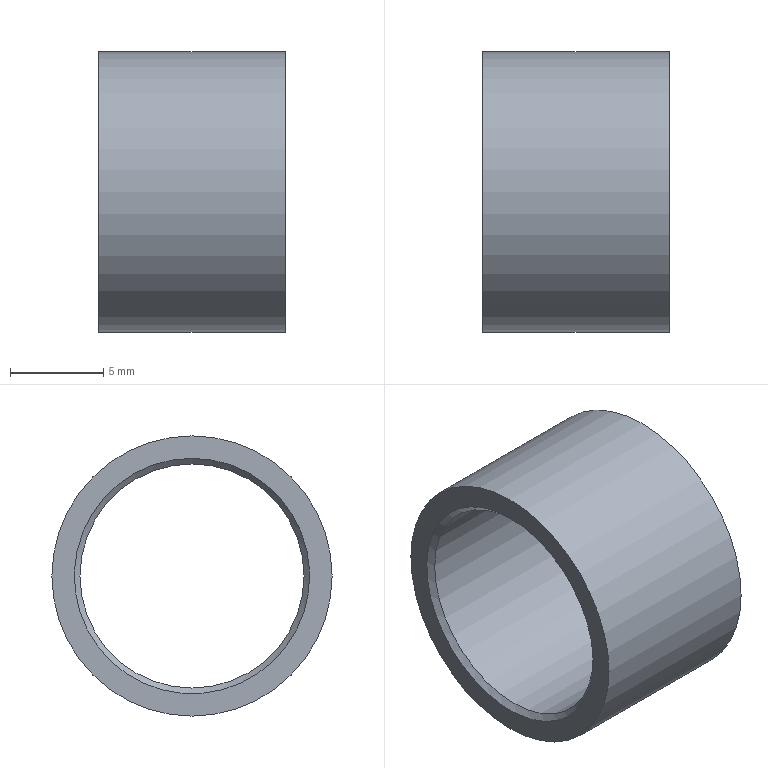Part | STEP file | 1 solid | 6 faces | box 10 x 15 x 15 mm | volume 632.723 mm3 | cylinder 2 | plane 2 | cone 2 | commonest cylinder face diameters 12 x1 15 x1
STEP:
#1=CARTESIAN_POINT('',(0.,0.,0.));
#2=DIRECTION('',(0.,0.,1.));
#3=DIRECTION('',(1.,0.,0.));
#4=AXIS2_PLACEMENT_3D('',#1,#2,#3);
#5=CARTESIAN_POINT('',(0.,0.,7.5));
#6=VERTEX_POINT('',#5);
#7=CARTESIAN_POINT('',(0.,0.,0.));
#8=DIRECTION('',(1.,0.,0.));
#9=DIRECTION('',(0.,0.,1.));
#10=AXIS2_PLACEMENT_3D('',#7,#8,#9);
#11=CIRCLE('',#10,7.5);
#12=CARTESIAN_POINT('',(0.,0.,0.));
#13=DIRECTION('',(-1.,0.,0.));
#14=DIRECTION('',(0.,0.,1.));
#15=AXIS2_PLACEMENT_3D('',#12,#13,#14);
#16=CYLINDRICAL_SURFACE('',#15,7.5);
#17=CARTESIAN_POINT('',(6.283,0.));
#18=DIRECTION('',(-1.,0.));
#19=VECTOR('',#18,1.);
#20=LINE('',#17,#19);
#21=(GEOMETRIC_REPRESENTATION_CONTEXT(2)PARAMETRIC_REPRESENTATION_CONTEXT()REPRESENTATION_CONTEXT('',''));
#22=DEFINITIONAL_REPRESENTATION('',(#20),#21);
#23=PCURVE('',#16,#22);
#24=CARTESIAN_POINT('',(0.,7.5,0.));
#25=DIRECTION('',(1.,0.,0.));
#26=DIRECTION('',(0.,0.,-1.));
#27=AXIS2_PLACEMENT_3D('',#24,#25,#26);
#28=PLANE('',#27);
#29=CARTESIAN_POINT('',(0.,-7.5));
#30=DIRECTION('',(-1.,0.));
#31=AXIS2_PLACEMENT_2D('',#29,#30);
#32=CIRCLE('',#31,7.5);
#33=(GEOMETRIC_REPRESENTATION_CONTEXT(2)PARAMETRIC_REPRESENTATION_CONTEXT()REPRESENTATION_CONTEXT('',''));
#34=DEFINITIONAL_REPRESENTATION('',(#32),#33);
#35=PCURVE('',#28,#34);
#36=SURFACE_CURVE('',#11,(#23,#35),.PCURVE_S1.);
#37=EDGE_CURVE('',#6,#6,#36,.T.);
#38=ORIENTED_EDGE('',*,*,#37,.T.);
#39=CARTESIAN_POINT('',(10.,0.,7.5));
#40=VERTEX_POINT('',#39);
#41=CARTESIAN_POINT('',(10.,0.,7.5));
#42=CARTESIAN_POINT('',(0.,0.,7.5));
#43=B_SPLINE_CURVE_WITH_KNOTS('',1,(#41,#42),.UNSPECIFIED.,.F.,.F.,(2,2),(-10.,0.),.PIECEWISE_BEZIER_KNOTS.);
#44=CARTESIAN_POINT('',(0.,0.));
#45=DIRECTION('',(0.,1.));
#46=VECTOR('',#45,1.);
#47=LINE('',#44,#46);
#48=(GEOMETRIC_REPRESENTATION_CONTEXT(2)PARAMETRIC_REPRESENTATION_CONTEXT()REPRESENTATION_CONTEXT('',''));
#49=DEFINITIONAL_REPRESENTATION('',(#47),#48);
#50=PCURVE('',#16,#49);
#51=CARTESIAN_POINT('',(6.283,0.));
#52=DIRECTION('',(0.,1.));
#53=VECTOR('',#52,1.);
#54=LINE('',#51,#53);
#55=(GEOMETRIC_REPRESENTATION_CONTEXT(2)PARAMETRIC_REPRESENTATION_CONTEXT()REPRESENTATION_CONTEXT('',''));
#56=DEFINITIONAL_REPRESENTATION('',(#54),#55);
#57=PCURVE('',#16,#56);
#58=SEAM_CURVE('',#43,(#50,#57),.PCURVE_S1.);
#59=EDGE_CURVE('',#40,#6,#58,.T.);
#60=ORIENTED_EDGE('',*,*,#59,.F.);
#61=CARTESIAN_POINT('',(10.,0.,0.));
#62=DIRECTION('',(-1.,0.,0.));
#63=DIRECTION('',(0.,0.,1.));
#64=AXIS2_PLACEMENT_3D('',#61,#62,#63);
#65=CIRCLE('',#64,7.5);
#66=CARTESIAN_POINT('',(0.,-10.));
#67=DIRECTION('',(1.,0.));
#68=VECTOR('',#67,1.);
#69=LINE('',#66,#68);
#70=(GEOMETRIC_REPRESENTATION_CONTEXT(2)PARAMETRIC_REPRESENTATION_CONTEXT()REPRESENTATION_CONTEXT('',''));
#71=DEFINITIONAL_REPRESENTATION('',(#69),#70);
#72=PCURVE('',#16,#71);
#73=CARTESIAN_POINT('',(10.,7.5,0.));
#74=DIRECTION('',(-1.,0.,0.));
#75=DIRECTION('',(0.,0.,1.));
#76=AXIS2_PLACEMENT_3D('',#73,#74,#75);
#77=PLANE('',#76);
#78=CARTESIAN_POINT('',(0.,-7.5));
#79=DIRECTION('',(1.,0.));
#80=AXIS2_PLACEMENT_2D('',#78,#79);
#81=CIRCLE('',#80,7.5);
#82=(GEOMETRIC_REPRESENTATION_CONTEXT(2)PARAMETRIC_REPRESENTATION_CONTEXT()REPRESENTATION_CONTEXT('',''));
#83=DEFINITIONAL_REPRESENTATION('',(#81),#82);
#84=PCURVE('',#77,#83);
#85=SURFACE_CURVE('',#65,(#72,#84),.PCURVE_S1.);
#86=EDGE_CURVE('',#40,#40,#85,.T.);
#87=ORIENTED_EDGE('',*,*,#86,.T.);
#88=ORIENTED_EDGE('',*,*,#59,.T.);
#89=EDGE_LOOP('',(#38,#60,#87,#88));
#90=FACE_BOUND('',#89,.T.);
#91=ADVANCED_FACE('',(#90),#16,.T.);
#92=CARTESIAN_POINT('',(0.,0.,6.3));
#93=VERTEX_POINT('',#92);
#94=CARTESIAN_POINT('',(0.,0.,0.));
#95=DIRECTION('',(-1.,0.,0.));
#96=DIRECTION('',(0.,0.,1.));
#97=AXIS2_PLACEMENT_3D('',#94,#95,#96);
#98=CIRCLE('',#97,6.3);
#99=CARTESIAN_POINT('',(-6.3,-7.5));
#100=CARTESIAN_POINT('',(-6.3,3.412));
#101=CARTESIAN_POINT('',(3.15,-2.044));
#102=CARTESIAN_POINT('',(12.6,-7.5));
#103=CARTESIAN_POINT('',(3.15,-12.956));
#104=CARTESIAN_POINT('',(-6.3,-18.412));
#105=CARTESIAN_POINT('',(-6.3,-7.5));
#106=(BOUNDED_CURVE()B_SPLINE_CURVE(2,(#99,#100,#101,#102,#103,#104,#105),.UNSPECIFIED.,.T.,.F.)B_SPLINE_CURVE_WITH_KNOTS((1,2,2,2,2,1),(-2.094,0.,2.094,4.189,6.283,8.378),.UNSPECIFIED.)CURVE()GEOMETRIC_REPRESENTATION_ITEM()RATIONAL_B_SPLINE_CURVE((1.,0.5,1.,0.5,1.,0.5,1.))REPRESENTATION_ITEM(''));
#107=(GEOMETRIC_REPRESENTATION_CONTEXT(2)PARAMETRIC_REPRESENTATION_CONTEXT()REPRESENTATION_CONTEXT('',''));
#108=DEFINITIONAL_REPRESENTATION('',(#106),#107);
#109=PCURVE('',#28,#108);
#110=CARTESIAN_POINT('',(0.,0.,0.));
#111=DIRECTION('',(-1.,0.,0.));
#112=DIRECTION('',(0.,0.,1.));
#113=AXIS2_PLACEMENT_3D('',#110,#111,#112);
#114=CONICAL_SURFACE('',#113,6.3,0.7854);
#115=CARTESIAN_POINT('',(0.,0.));
#116=DIRECTION('',(1.,0.));
#117=VECTOR('',#116,1.);
#118=LINE('',#115,#117);
#119=(GEOMETRIC_REPRESENTATION_CONTEXT(2)PARAMETRIC_REPRESENTATION_CONTEXT()REPRESENTATION_CONTEXT('',''));
#120=DEFINITIONAL_REPRESENTATION('',(#118),#119);
#121=PCURVE('',#114,#120);
#122=SURFACE_CURVE('',#98,(#109,#121),.PCURVE_S1.);
#123=EDGE_CURVE('',#93,#93,#122,.T.);
#124=ORIENTED_EDGE('',*,*,#123,.F.);
#125=EDGE_LOOP('',(#124));
#126=FACE_BOUND('',#125,.T.);
#127=ORIENTED_EDGE('',*,*,#37,.F.);
#128=EDGE_LOOP('',(#127));
#129=FACE_BOUND('',#128,.T.);
#130=ADVANCED_FACE('',(#126,#129),#28,.F.);
#131=CARTESIAN_POINT('',(10.,0.,-6.3));
#132=VERTEX_POINT('',#131);
#133=CARTESIAN_POINT('',(10.,0.,0.));
#134=DIRECTION('',(1.,0.,0.));
#135=DIRECTION('',(0.,0.,-1.));
#136=AXIS2_PLACEMENT_3D('',#133,#134,#135);
#137=CIRCLE('',#136,6.3);
#138=CARTESIAN_POINT('',(-6.3,-7.5));
#139=CARTESIAN_POINT('',(-6.3,3.412));
#140=CARTESIAN_POINT('',(3.15,-2.044));
#141=CARTESIAN_POINT('',(12.6,-7.5));
#142=CARTESIAN_POINT('',(3.15,-12.956));
#143=CARTESIAN_POINT('',(-6.3,-18.412));
#144=CARTESIAN_POINT('',(-6.3,-7.5));
#145=(BOUNDED_CURVE()B_SPLINE_CURVE(2,(#138,#139,#140,#141,#142,#143,#144),.UNSPECIFIED.,.T.,.F.)B_SPLINE_CURVE_WITH_KNOTS((1,2,2,2,2,1),(-2.094,0.,2.094,4.189,6.283,8.378),.UNSPECIFIED.)CURVE()GEOMETRIC_REPRESENTATION_ITEM()RATIONAL_B_SPLINE_CURVE((1.,0.5,1.,0.5,1.,0.5,1.))REPRESENTATION_ITEM(''));
#146=(GEOMETRIC_REPRESENTATION_CONTEXT(2)PARAMETRIC_REPRESENTATION_CONTEXT()REPRESENTATION_CONTEXT('',''));
#147=DEFINITIONAL_REPRESENTATION('',(#145),#146);
#148=PCURVE('',#77,#147);
#149=CARTESIAN_POINT('',(10.,0.,0.));
#150=DIRECTION('',(1.,0.,0.));
#151=DIRECTION('',(0.,0.,-1.));
#152=AXIS2_PLACEMENT_3D('',#149,#150,#151);
#153=CONICAL_SURFACE('',#152,6.3,0.7854);
#154=CARTESIAN_POINT('',(0.,0.));
#155=DIRECTION('',(1.,0.));
#156=VECTOR('',#155,1.);
#157=LINE('',#154,#156);
#158=(GEOMETRIC_REPRESENTATION_CONTEXT(2)PARAMETRIC_REPRESENTATION_CONTEXT()REPRESENTATION_CONTEXT('',''));
#159=DEFINITIONAL_REPRESENTATION('',(#157),#158);
#160=PCURVE('',#153,#159);
#161=SURFACE_CURVE('',#137,(#148,#160),.PCURVE_S1.);
#162=EDGE_CURVE('',#132,#132,#161,.T.);
#163=ORIENTED_EDGE('',*,*,#162,.F.);
#164=EDGE_LOOP('',(#163));
#165=FACE_BOUND('',#164,.T.);
#166=ORIENTED_EDGE('',*,*,#86,.F.);
#167=EDGE_LOOP('',(#166));
#168=FACE_BOUND('',#167,.T.);
#169=ADVANCED_FACE('',(#165,#168),#77,.F.);
#170=ORIENTED_EDGE('',*,*,#123,.F.);
#171=CARTESIAN_POINT('',(0.3,0.,6.));
#172=VERTEX_POINT('',#171);
#173=CARTESIAN_POINT('',(0.3,0.,6.));
#174=CARTESIAN_POINT('',(0.,0.,6.3));
#175=B_SPLINE_CURVE_WITH_KNOTS('',1,(#173,#174),.UNSPECIFIED.,.F.,.F.,(2,2),(-0.4243,0.),.PIECEWISE_BEZIER_KNOTS.);
#176=CARTESIAN_POINT('',(0.,0.));
#177=DIRECTION('',(0.,1.));
#178=VECTOR('',#177,1.);
#179=LINE('',#176,#178);
#180=(GEOMETRIC_REPRESENTATION_CONTEXT(2)PARAMETRIC_REPRESENTATION_CONTEXT()REPRESENTATION_CONTEXT('',''));
#181=DEFINITIONAL_REPRESENTATION('',(#179),#180);
#182=PCURVE('',#114,#181);
#183=CARTESIAN_POINT('',(6.283,0.));
#184=DIRECTION('',(0.,1.));
#185=VECTOR('',#184,1.);
#186=LINE('',#183,#185);
#187=(GEOMETRIC_REPRESENTATION_CONTEXT(2)PARAMETRIC_REPRESENTATION_CONTEXT()REPRESENTATION_CONTEXT('',''));
#188=DEFINITIONAL_REPRESENTATION('',(#186),#187);
#189=PCURVE('',#114,#188);
#190=SEAM_CURVE('',#175,(#182,#189),.PCURVE_S1.);
#191=EDGE_CURVE('',#172,#93,#190,.T.);
#192=ORIENTED_EDGE('',*,*,#191,.F.);
#193=CARTESIAN_POINT('',(0.3,0.,0.));
#194=DIRECTION('',(-1.,0.,0.));
#195=DIRECTION('',(0.,0.,1.));
#196=AXIS2_PLACEMENT_3D('',#193,#194,#195);
#197=CIRCLE('',#196,6.);
#198=CARTESIAN_POINT('',(0.,-0.3));
#199=DIRECTION('',(1.,0.));
#200=VECTOR('',#199,1.);
#201=LINE('',#198,#200);
#202=(GEOMETRIC_REPRESENTATION_CONTEXT(2)PARAMETRIC_REPRESENTATION_CONTEXT()REPRESENTATION_CONTEXT('',''));
#203=DEFINITIONAL_REPRESENTATION('',(#201),#202);
#204=PCURVE('',#114,#203);
#205=CARTESIAN_POINT('',(0.,0.,0.));
#206=DIRECTION('',(-1.,0.,0.));
#207=DIRECTION('',(0.,0.,1.));
#208=AXIS2_PLACEMENT_3D('',#205,#206,#207);
#209=CYLINDRICAL_SURFACE('',#208,6.);
#210=CARTESIAN_POINT('',(0.,-0.3));
#211=DIRECTION('',(1.,0.));
#212=VECTOR('',#211,1.);
#213=LINE('',#210,#212);
#214=(GEOMETRIC_REPRESENTATION_CONTEXT(2)PARAMETRIC_REPRESENTATION_CONTEXT()REPRESENTATION_CONTEXT('',''));
#215=DEFINITIONAL_REPRESENTATION('',(#213),#214);
#216=PCURVE('',#209,#215);
#217=SURFACE_CURVE('',#197,(#204,#216),.PCURVE_S1.);
#218=EDGE_CURVE('',#172,#172,#217,.T.);
#219=ORIENTED_EDGE('',*,*,#218,.T.);
#220=ORIENTED_EDGE('',*,*,#191,.T.);
#221=EDGE_LOOP('',(#170,#192,#219,#220));
#222=FACE_BOUND('',#221,.F.);
#223=ADVANCED_FACE('',(#222),#114,.F.);
#224=ORIENTED_EDGE('',*,*,#162,.F.);
#225=CARTESIAN_POINT('',(9.7,0.,-6.));
#226=VERTEX_POINT('',#225);
#227=CARTESIAN_POINT('',(9.7,0.,-6.));
#228=CARTESIAN_POINT('',(10.,0.,-6.3));
#229=B_SPLINE_CURVE_WITH_KNOTS('',1,(#227,#228),.UNSPECIFIED.,.F.,.F.,(2,2),(-0.4243,0.),.PIECEWISE_BEZIER_KNOTS.);
#230=CARTESIAN_POINT('',(0.,0.));
#231=DIRECTION('',(0.,1.));
#232=VECTOR('',#231,1.);
#233=LINE('',#230,#232);
#234=(GEOMETRIC_REPRESENTATION_CONTEXT(2)PARAMETRIC_REPRESENTATION_CONTEXT()REPRESENTATION_CONTEXT('',''));
#235=DEFINITIONAL_REPRESENTATION('',(#233),#234);
#236=PCURVE('',#153,#235);
#237=CARTESIAN_POINT('',(6.283,0.));
#238=DIRECTION('',(0.,1.));
#239=VECTOR('',#238,1.);
#240=LINE('',#237,#239);
#241=(GEOMETRIC_REPRESENTATION_CONTEXT(2)PARAMETRIC_REPRESENTATION_CONTEXT()REPRESENTATION_CONTEXT('',''));
#242=DEFINITIONAL_REPRESENTATION('',(#240),#241);
#243=PCURVE('',#153,#242);
#244=SEAM_CURVE('',#229,(#236,#243),.PCURVE_S1.);
#245=EDGE_CURVE('',#226,#132,#244,.T.);
#246=ORIENTED_EDGE('',*,*,#245,.F.);
#247=CARTESIAN_POINT('',(9.7,0.,6.));
#248=VERTEX_POINT('',#247);
#249=CARTESIAN_POINT('',(9.7,0.,0.));
#250=DIRECTION('',(1.,0.,0.));
#251=DIRECTION('',(0.,0.,-1.));
#252=AXIS2_PLACEMENT_3D('',#249,#250,#251);
#253=CIRCLE('',#252,6.);
#254=CARTESIAN_POINT('',(0.,-0.3));
#255=DIRECTION('',(1.,0.));
#256=VECTOR('',#255,1.);
#257=LINE('',#254,#256);
#258=(GEOMETRIC_REPRESENTATION_CONTEXT(2)PARAMETRIC_REPRESENTATION_CONTEXT()REPRESENTATION_CONTEXT('',''));
#259=DEFINITIONAL_REPRESENTATION('',(#257),#258);
#260=PCURVE('',#153,#259);
#261=CARTESIAN_POINT('',(3.142,-9.7));
#262=DIRECTION('',(-1.,0.));
#263=VECTOR('',#262,1.);
#264=LINE('',#261,#263);
#265=(GEOMETRIC_REPRESENTATION_CONTEXT(2)PARAMETRIC_REPRESENTATION_CONTEXT()REPRESENTATION_CONTEXT('',''));
#266=DEFINITIONAL_REPRESENTATION('',(#264),#265);
#267=PCURVE('',#209,#266);
#268=SURFACE_CURVE('',#253,(#260,#267),.PCURVE_S1.);
#269=EDGE_CURVE('',#226,#248,#268,.T.);
#270=ORIENTED_EDGE('',*,*,#269,.T.);
#271=CARTESIAN_POINT('',(9.7,0.,0.));
#272=DIRECTION('',(1.,0.,0.));
#273=DIRECTION('',(0.,0.,-1.));
#274=AXIS2_PLACEMENT_3D('',#271,#272,#273);
#275=CIRCLE('',#274,6.);
#276=CARTESIAN_POINT('',(0.,-0.3));
#277=DIRECTION('',(1.,0.));
#278=VECTOR('',#277,1.);
#279=LINE('',#276,#278);
#280=(GEOMETRIC_REPRESENTATION_CONTEXT(2)PARAMETRIC_REPRESENTATION_CONTEXT()REPRESENTATION_CONTEXT('',''));
#281=DEFINITIONAL_REPRESENTATION('',(#279),#280);
#282=PCURVE('',#153,#281);
#283=CARTESIAN_POINT('',(9.425,-9.7));
#284=DIRECTION('',(-1.,0.));
#285=VECTOR('',#284,1.);
#286=LINE('',#283,#285);
#287=(GEOMETRIC_REPRESENTATION_CONTEXT(2)PARAMETRIC_REPRESENTATION_CONTEXT()REPRESENTATION_CONTEXT('',''));
#288=DEFINITIONAL_REPRESENTATION('',(#286),#287);
#289=PCURVE('',#209,#288);
#290=SURFACE_CURVE('',#275,(#282,#289),.PCURVE_S1.);
#291=EDGE_CURVE('',#248,#226,#290,.T.);
#292=ORIENTED_EDGE('',*,*,#291,.T.);
#293=ORIENTED_EDGE('',*,*,#245,.T.);
#294=EDGE_LOOP('',(#224,#246,#270,#292,#293));
#295=FACE_BOUND('',#294,.F.);
#296=ADVANCED_FACE('',(#295),#153,.F.);
#297=ORIENTED_EDGE('',*,*,#218,.F.);
#298=CARTESIAN_POINT('',(9.7,0.,6.));
#299=CARTESIAN_POINT('',(0.3,0.,6.));
#300=B_SPLINE_CURVE_WITH_KNOTS('',1,(#298,#299),.UNSPECIFIED.,.F.,.F.,(2,2),(-9.7,-0.3),.PIECEWISE_BEZIER_KNOTS.);
#301=CARTESIAN_POINT('',(0.,0.));
#302=DIRECTION('',(0.,1.));
#303=VECTOR('',#302,1.);
#304=LINE('',#301,#303);
#305=(GEOMETRIC_REPRESENTATION_CONTEXT(2)PARAMETRIC_REPRESENTATION_CONTEXT()REPRESENTATION_CONTEXT('',''));
#306=DEFINITIONAL_REPRESENTATION('',(#304),#305);
#307=PCURVE('',#209,#306);
#308=CARTESIAN_POINT('',(6.283,0.));
#309=DIRECTION('',(0.,1.));
#310=VECTOR('',#309,1.);
#311=LINE('',#308,#310);
#312=(GEOMETRIC_REPRESENTATION_CONTEXT(2)PARAMETRIC_REPRESENTATION_CONTEXT()REPRESENTATION_CONTEXT('',''));
#313=DEFINITIONAL_REPRESENTATION('',(#311),#312);
#314=PCURVE('',#209,#313);
#315=SEAM_CURVE('',#300,(#307,#314),.PCURVE_S1.);
#316=EDGE_CURVE('',#248,#172,#315,.T.);
#317=ORIENTED_EDGE('',*,*,#316,.F.);
#318=ORIENTED_EDGE('',*,*,#269,.F.);
#319=ORIENTED_EDGE('',*,*,#291,.F.);
#320=ORIENTED_EDGE('',*,*,#316,.T.);
#321=EDGE_LOOP('',(#297,#317,#318,#319,#320));
#322=FACE_BOUND('',#321,.F.);
#323=ADVANCED_FACE('',(#322),#209,.F.);
#324=CLOSED_SHELL('',(#91,#130,#169,#223,#296,#323));
#325=MANIFOLD_SOLID_BREP('',#324);
#326=(LENGTH_UNIT()NAMED_UNIT(*)SI_UNIT(.MILLI.,.METRE.));
#327=UNCERTAINTY_MEASURE_WITH_UNIT(LENGTH_MEASURE(0.00001),#326,'','');
#328=(NAMED_UNIT(*)PLANE_ANGLE_UNIT()SI_UNIT($,.RADIAN.));
#329=(NAMED_UNIT(*)SI_UNIT($,.STERADIAN.)SOLID_ANGLE_UNIT());
#330=(GEOMETRIC_REPRESENTATION_CONTEXT(3)GLOBAL_UNCERTAINTY_ASSIGNED_CONTEXT((#327))GLOBAL_UNIT_ASSIGNED_CONTEXT((#326,#328,#329))REPRESENTATION_CONTEXT('',''));
#331=ADVANCED_BREP_SHAPE_REPRESENTATION('',(#4,#325),#330);